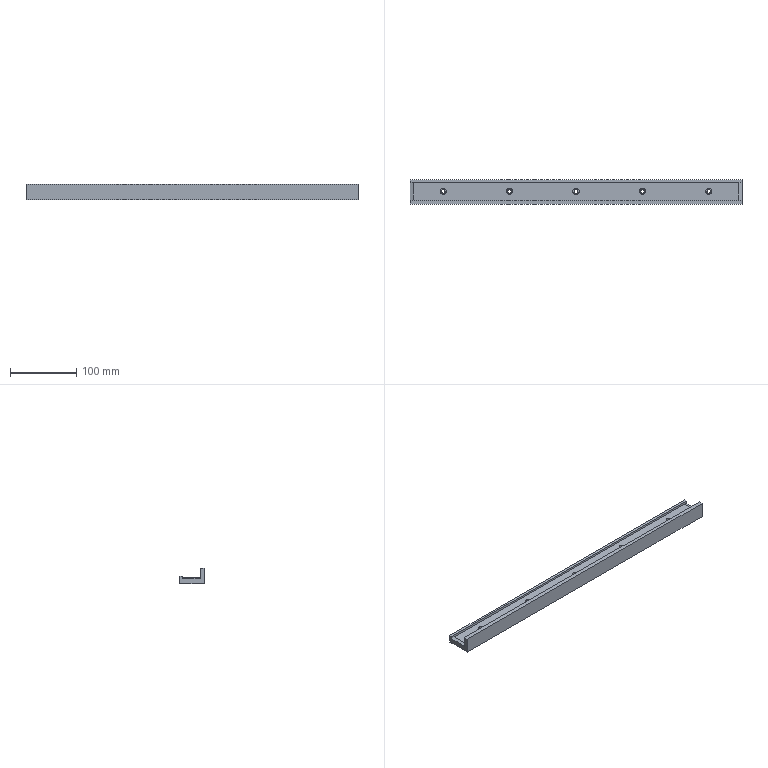Part | STEP file | CON-016 | 1 solid | 37 faces | box 500 x 37 x 24 mm | volume 214836 mm3 | cylinder 20 | plane 17 | commonest cylinder face diameters 5.5 x10 9.5 x10